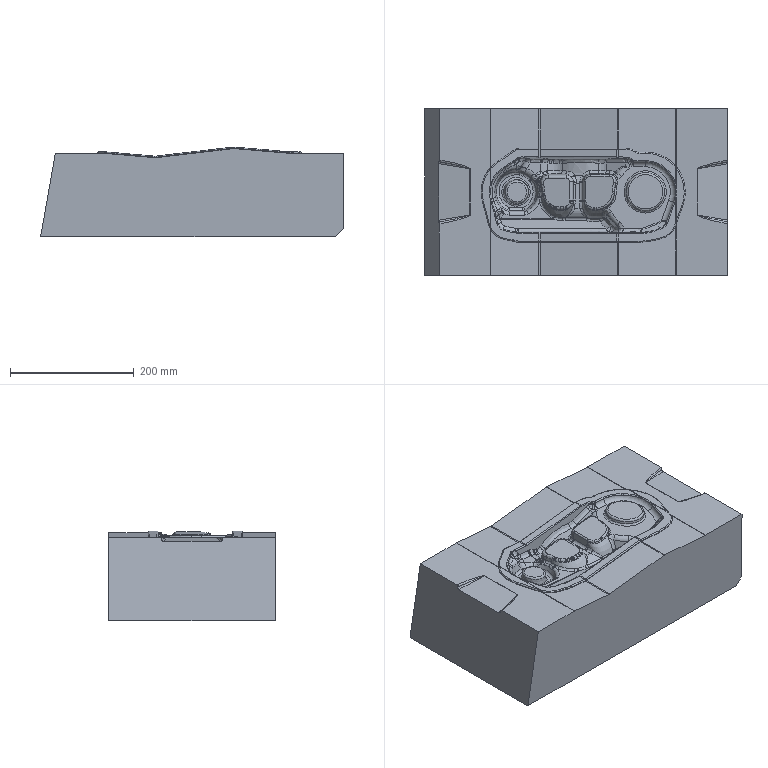CAM job | NX | 3-axis milling | part box 490.523 x 270 x 145.452 mm
Tools:
number,name,description,diameter,corner_radius,flute_length,length,flutes
0,25.,Milling Tool-5 Parameters,25.0,0.8,50.0,75.0,2
0,16R0.8,Milling Tool-5 Parameters,16.0,0.8,50.0,75.0,2
0,B8,Milling Tool-Ball Mill,8.0,4.0,50.0,75.0,2
0,6.,Milling Tool-Ball Mill,6.0,3.0,50.0,75.0,2
Operations:
program,operation,operation_type,tool,method,geometry_group,spindle_rpm,surface_speed,feed_per_tooth,feed_cut,feed_plunge,cut_length_mm,path_length_mm,cut_time_min,machine_time_min
ROUGHING,ZLEVEL_PROFILE,ZLevelMilling,25.,METHOD,MCS_MILL,3000.0,282.0,0.4167,2500.0,100.0,79843.36,80162.061,31.937,31.969
ROUGHING,CAVITY_MILL,CavityMilling,25.,METHOD,WORKPIECE,3000.0,282.0,0.4167,2500.0,100.0,212520.524,219819.346,85.008,85.738
参考刀具,CAVITY_MILL_1,CavityMilling,16R0.8,METHOD,WORKPIECE,3000.0,282.0,0.4167,2500.0,100.0,85459.751,116294.88,34.184,37.267
PROGRAM_2,ZLEVEL_PROFILE_1,ZLevelMilling,B8,METHOD,WORKPIECE,3000.0,282.0,0.4167,2500.0,100.0,75528.496,122825.175,30.211,34.941
FINISH,FIXED_CONTOUR,SurfaceContour,6.,METHOD,WORKPIECE,3000.0,282.0,0.4167,2500.0,100.0,709108.109,732950.101,283.643,286.027